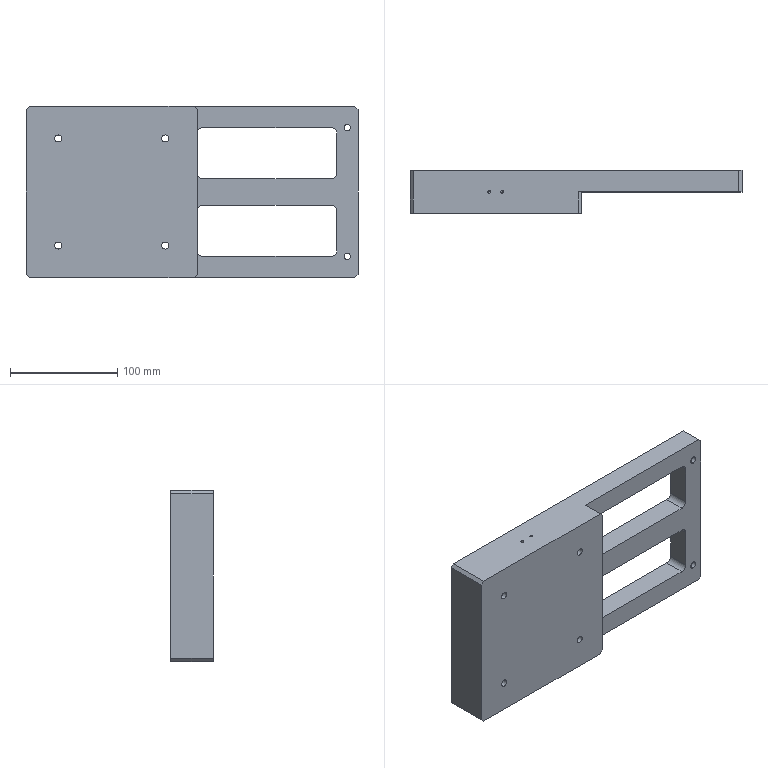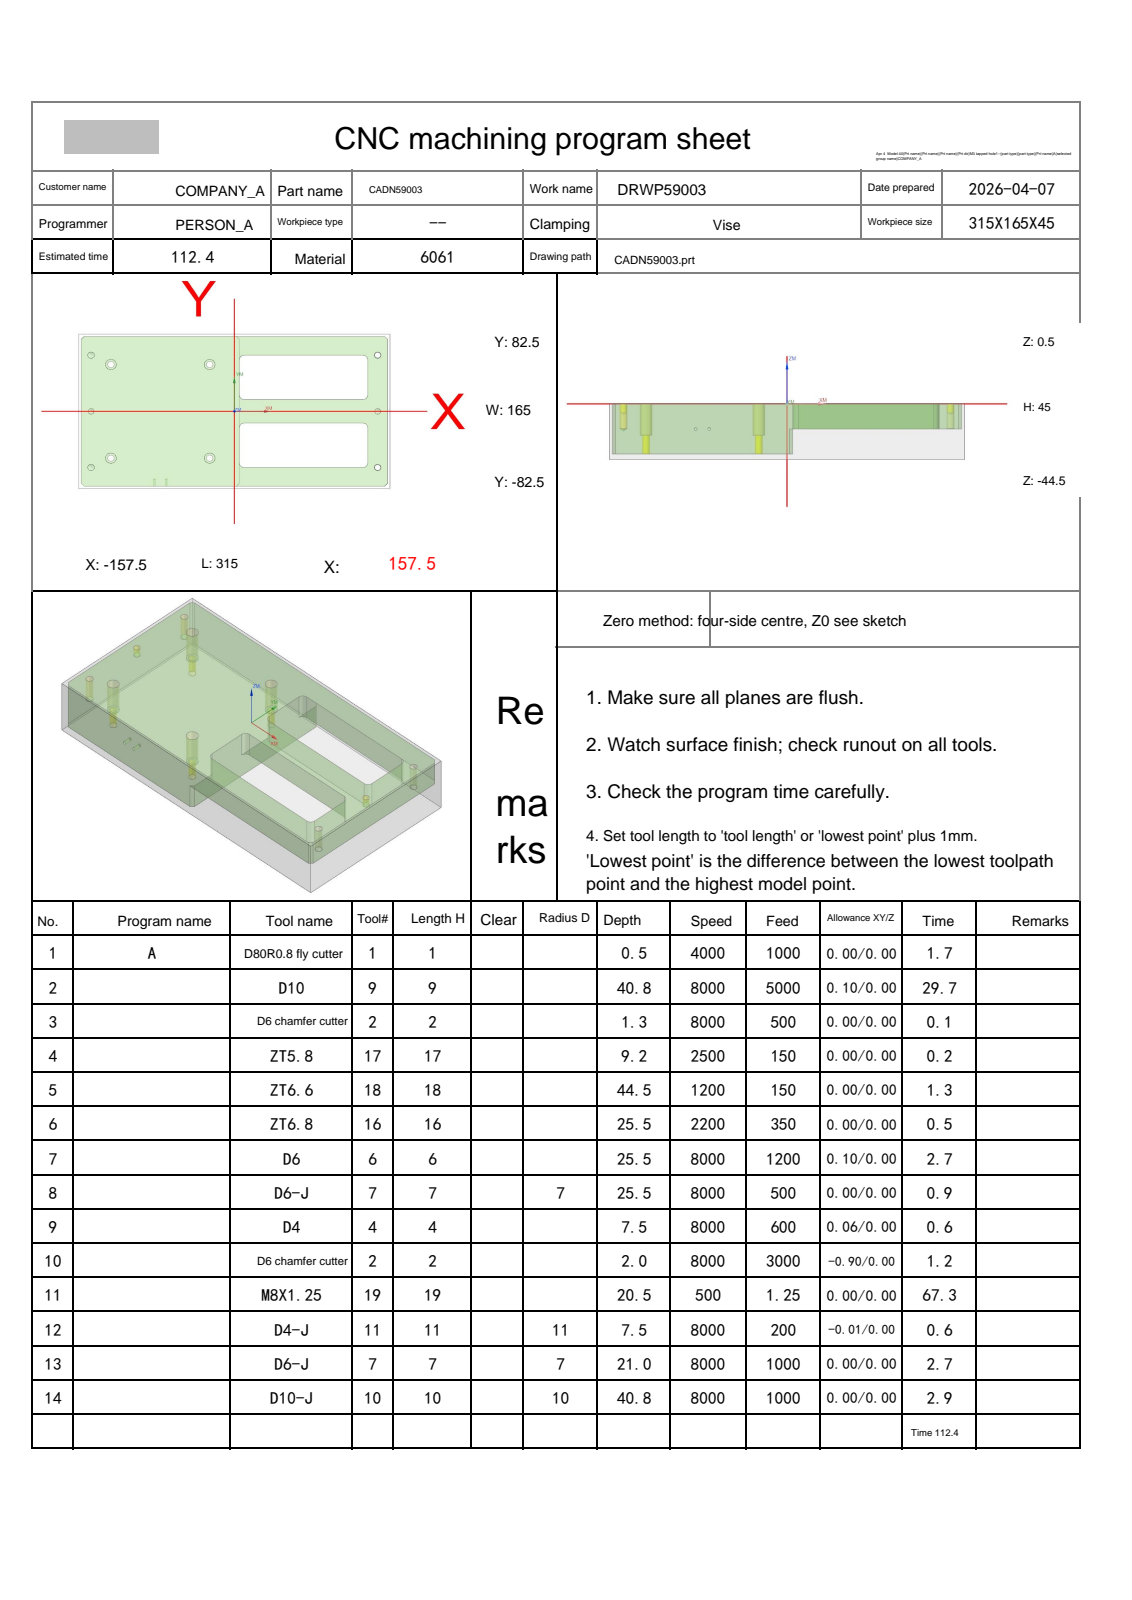NC program | NX | posted by the shop | part box 310 x 40 x 160 mm
Lines 4354 to 5464 of 5464:
N3 T02 M06
(D6 chamfer cutter  D=6. R=0. H=02 ce=0.00 di=0.10)
G00 G90 G54 X-145. Y-60. M03 S8000
G43 H02 Z20.
M08
G98 G81 X-145. Y-60. Z-.8 R1. F500.
X-125. Y-50.
X-145. Y0.0
Y60.
X-125. Y50.
X-25.
Y-50.
X145. Y-60.
Y0.0
Y60.
G80
G00 Z20.
G91 G28 Z0.0
M05
M09
G91 G28 Z0.0
M01
N4 T17 M06
(ZT5.8 D=5.8 DR_a=118 H=17)
G00 G90 G54 X-145. Y0.0 M03 S2500
G43 H17 Z20.
M08
G98 G83 X-145. Y0.0 Z-8.703 R1. F150. Q2.
X145.
G80
G00 Z20.
G91 G28 Z0.0
M05
M09
G91 G28 Z0.0
M01
N5 T18 M06
(ZT6.6 D=6.6 DR_a=118 H=18)
G00 G90 G54 X-25. Y50. M03 S1200
G43 H18 Z20.
M08
G98 G83 X-25. Y50. Z-43.983 R1. F150. Q2.
X-125.
Y-50.
X-25.
G80
G00 Z20.
G91 G28 Z0.0
M05
M09
G91 G28 Z0.0
M01
N6 T16 M06
(ZT6.8 D=6.8 DR_a=118 H=16)
G00 G90 G54 X-145. Y60. M03 S2200
G43 H16 Z20.
M08
G98 G83 X-145. Y60. Z-25. R1. F150. Q2.
Y-60.
G80
G00 Z20.
G00 G90 X145. Y-60. M03 S1800
Z20.
G98 G83 X145. Y-60. Z-25. R1. F350. Q3.
Y60.
G80
G00 Z20.
G91 G28 Z0.0
M05
M09
G91 G28 Z0.0
M01
N7 T06 M06
(D6  D=6. R=0. H=06 ce=0.10 di=0.00)
G00 G90 G54 X-25. Y50. M03 S8000
G43 H06 Z20.
M08
Z.5
G03 X-23.8 Y48.8 I1.2 J0.0 F1200.
X-22.6 Y50. I0.0 J1.2
X-22.6 Y50. Z0.0 I-2.4 J0.0
X-22.6 Y50. Z-.5 I-2.4 J0.0
X-22.6 Y50. Z-1. I-2.4 J0.0
X-22.6 Y50. Z-1.5 I-2.4 J0.0
X-22.6 Y50. Z-2. I-2.4 J0.0
X-22.6 Y50. Z-2.5 I-2.4 J0.0
X-22.6 Y50. Z-3. I-2.4 J0.0
X-22.6 Y50. Z-3.5 I-2.4 J0.0
X-22.6 Y50. Z-4. I-2.4 J0.0
X-22.6 Y50. Z-4.5 I-2.4 J0.0
X-22.6 Y50. Z-5. I-2.4 J0.0
X-22.6 Y50. Z-5.5 I-2.4 J0.0
X-22.6 Y50. Z-6. I-2.4 J0.0
X-22.6 Y50. Z-6.5 I-2.4 J0.0
X-22.6 Y50. Z-7. I-2.4 J0.0
X-22.6 Y50. Z-7.5 I-2.4 J0.0
X-22.6 Y50. Z-8. I-2.4 J0.0
X-22.6 Y50. Z-8.5 I-2.4 J0.0
X-22.6 Y50. Z-9. I-2.4 J0.0
X-22.6 Y50. Z-9.5 I-2.4 J0.0
X-22.6 Y50. Z-10. I-2.4 J0.0
X-22.6 Y50. Z-10.5 I-2.4 J0.0
X-22.6 Y50. Z-11. I-2.4 J0.0
X-22.6 Y50. Z-11.5 I-2.4 J0.0
X-22.6 Y50. Z-12. I-2.4 J0.0
X-22.6 Y50. Z-12.5 I-2.4 J0.0
X-22.6 Y50. Z-13. I-2.4 J0.0
X-22.6 Y50. Z-13.5 I-2.4 J0.0
X-22.6 Y50. Z-14. I-2.4 J0.0
X-22.6 Y50. Z-14.5 I-2.4 J0.0
X-22.6 Y50. Z-15. I-2.4 J0.0
X-22.6 Y50. Z-15.5 I-2.4 J0.0
X-22.6 Y50. Z-16. I-2.4 J0.0
X-22.6 Y50. Z-16.5 I-2.4 J0.0
X-22.6 Y50. Z-17. I-2.4 J0.0
X-22.6 Y50. Z-17.5 I-2.4 J0.0
X-22.6 Y50. Z-18. I-2.4 J0.0
X-22.6 Y50. Z-18.5 I-2.4 J0.0
X-22.6 Y50. Z-19. I-2.4 J0.0
X-22.6 Y50. Z-19.5 I-2.4 J0.0
X-22.6 Y50. Z-20. I-2.4 J0.0
X-22.6 Y50. Z-20.5 I-2.4 J0.0
X-22.6 Y50. Z-21. I-2.4 J0.0
X-22.6 Y50. Z-21.5 I-2.4 J0.0
X-22.6 Y50. Z-22. I-2.4 J0.0
X-22.6 Y50. Z-22.5 I-2.4 J0.0
X-22.6 Y50. Z-23. I-2.4 J0.0
X-22.6 Y50. Z-23.5 I-2.4 J0.0
X-22.6 Y50. Z-24. I-2.4 J0.0
X-22.6 Y50. Z-24.5 I-2.4 J0.0
X-22.6 Y50. Z-25. I-2.4 J0.0
X-25. Y52.4 I-2.4 J0.0
X-27.4 Y50. I0.0 J-2.4
X-25. Y47.6 I2.4 J0.0
X-22.6 Y50. I0.0 J2.4
X-23.8 Y51.2 I-1.2 J0.0
X-25. Y50. I0.0 J-1.2
G00 Z20.
X-125.
Z.5
G03 X-123.8 Y48.8 I1.2 J0.0
X-122.6 Y50. I0.0 J1.2
X-122.6 Y50. Z0.0 I-2.4 J0.0
X-122.6 Y50. Z-.5 I-2.4 J0.0
X-122.6 Y50. Z-1. I-2.4 J0.0
X-122.6 Y50. Z-1.5 I-2.4 J0.0
X-122.6 Y50. Z-2. I-2.4 J0.0
X-122.6 Y50. Z-2.5 I-2.4 J0.0
X-122.6 Y50. Z-3. I-2.4 J0.0
X-122.6 Y50. Z-3.5 I-2.4 J0.0
X-122.6 Y50. Z-4. I-2.4 J0.0
X-122.6 Y50. Z-4.5 I-2.4 J0.0
X-122.6 Y50. Z-5. I-2.4 J0.0
X-122.6 Y50. Z-5.5 I-2.4 J0.0
X-122.6 Y50. Z-6. I-2.4 J0.0
X-122.6 Y50. Z-6.5 I-2.4 J0.0
X-122.6 Y50. Z-7. I-2.4 J0.0
X-122.6 Y50. Z-7.5 I-2.4 J0.0
X-122.6 Y50. Z-8. I-2.4 J0.0
X-122.6 Y50. Z-8.5 I-2.4 J0.0
X-122.6 Y50. Z-9. I-2.4 J0.0
X-122.6 Y50. Z-9.5 I-2.4 J0.0
X-122.6 Y50. Z-10. I-2.4 J0.0
X-122.6 Y50. Z-10.5 I-2.4 J0.0
X-122.6 Y50. Z-11. I-2.4 J0.0
X-122.6 Y50. Z-11.5 I-2.4 J0.0
X-122.6 Y50. Z-12. I-2.4 J0.0
X-122.6 Y50. Z-12.5 I-2.4 J0.0
X-122.6 Y50. Z-13. I-2.4 J0.0
X-122.6 Y50. Z-13.5 I-2.4 J0.0
X-122.6 Y50. Z-14. I-2.4 J0.0
X-122.6 Y50. Z-14.5 I-2.4 J0.0
X-122.6 Y50. Z-15. I-2.4 J0.0
X-122.6 Y50. Z-15.5 I-2.4 J0.0
X-122.6 Y50. Z-16. I-2.4 J0.0
X-122.6 Y50. Z-16.5 I-2.4 J0.0
X-122.6 Y50. Z-17. I-2.4 J0.0
X-122.6 Y50. Z-17.5 I-2.4 J0.0
X-122.6 Y50. Z-18. I-2.4 J0.0
X-122.6 Y50. Z-18.5 I-2.4 J0.0
X-122.6 Y50. Z-19. I-2.4 J0.0
X-122.6 Y50. Z-19.5 I-2.4 J0.0
X-122.6 Y50. Z-20. I-2.4 J0.0
X-122.6 Y50. Z-20.5 I-2.4 J0.0
X-122.6 Y50. Z-21. I-2.4 J0.0
X-122.6 Y50. Z-21.5 I-2.4 J0.0
X-122.6 Y50. Z-22. I-2.4 J0.0
X-122.6 Y50. Z-22.5 I-2.4 J0.0
X-122.6 Y50. Z-23. I-2.4 J0.0
X-122.6 Y50. Z-23.5 I-2.4 J0.0
X-122.6 Y50. Z-24. I-2.4 J0.0
X-122.6 Y50. Z-24.5 I-2.4 J0.0
X-122.6 Y50. Z-25. I-2.4 J0.0
X-125. Y52.4 I-2.4 J0.0
X-127.4 Y50. I0.0 J-2.4
X-125. Y47.6 I2.4 J0.0
X-122.6 Y50. I0.0 J2.4
X-123.8 Y51.2 I-1.2 J0.0
X-125. Y50. I0.0 J-1.2
G00 Z20.
Y-50.
Z.5
G03 X-123.8 Y-51.2 I1.2 J0.0
X-122.6 Y-50. I0.0 J1.2
X-122.6 Y-50. Z0.0 I-2.4 J0.0
X-122.6 Y-50. Z-.5 I-2.4 J0.0
X-122.6 Y-50. Z-1. I-2.4 J0.0
X-122.6 Y-50. Z-1.5 I-2.4 J0.0
X-122.6 Y-50. Z-2. I-2.4 J0.0
X-122.6 Y-50. Z-2.5 I-2.4 J0.0
X-122.6 Y-50. Z-3. I-2.4 J0.0
X-122.6 Y-50. Z-3.5 I-2.4 J0.0
X-122.6 Y-50. Z-4. I-2.4 J0.0
X-122.6 Y-50. Z-4.5 I-2.4 J0.0
X-122.6 Y-50. Z-5. I-2.4 J0.0
X-122.6 Y-50. Z-5.5 I-2.4 J0.0
X-122.6 Y-50. Z-6. I-2.4 J0.0
X-122.6 Y-50. Z-6.5 I-2.4 J0.0
X-122.6 Y-50. Z-7. I-2.4 J0.0
X-122.6 Y-50. Z-7.5 I-2.4 J0.0
X-122.6 Y-50. Z-8. I-2.4 J0.0
X-122.6 Y-50. Z-8.5 I-2.4 J0.0
X-122.6 Y-50. Z-9. I-2.4 J0.0
X-122.6 Y-50. Z-9.5 I-2.4 J0.0
X-122.6 Y-50. Z-10. I-2.4 J0.0
X-122.6 Y-50. Z-10.5 I-2.4 J0.0
X-122.6 Y-50. Z-11. I-2.4 J0.0
X-122.6 Y-50. Z-11.5 I-2.4 J0.0
X-122.6 Y-50. Z-12. I-2.4 J0.0
X-122.6 Y-50. Z-12.5 I-2.4 J0.0
X-122.6 Y-50. Z-13. I-2.4 J0.0
X-122.6 Y-50. Z-13.5 I-2.4 J0.0
X-122.6 Y-50. Z-14. I-2.4 J0.0
X-122.6 Y-50. Z-14.5 I-2.4 J0.0
X-122.6 Y-50. Z-15. I-2.4 J0.0
X-122.6 Y-50. Z-15.5 I-2.4 J0.0
X-122.6 Y-50. Z-16. I-2.4 J0.0
X-122.6 Y-50. Z-16.5 I-2.4 J0.0
X-122.6 Y-50. Z-17. I-2.4 J0.0
X-122.6 Y-50. Z-17.5 I-2.4 J0.0
X-122.6 Y-50. Z-18. I-2.4 J0.0
X-122.6 Y-50. Z-18.5 I-2.4 J0.0
X-122.6 Y-50. Z-19. I-2.4 J0.0
X-122.6 Y-50. Z-19.5 I-2.4 J0.0
X-122.6 Y-50. Z-20. I-2.4 J0.0
X-122.6 Y-50. Z-20.5 I-2.4 J0.0
X-122.6 Y-50. Z-21. I-2.4 J0.0
X-122.6 Y-50. Z-21.5 I-2.4 J0.0
X-122.6 Y-50. Z-22. I-2.4 J0.0
X-122.6 Y-50. Z-22.5 I-2.4 J0.0
X-122.6 Y-50. Z-23. I-2.4 J0.0
X-122.6 Y-50. Z-23.5 I-2.4 J0.0
X-122.6 Y-50. Z-24. I-2.4 J0.0
X-122.6 Y-50. Z-24.5 I-2.4 J0.0
X-122.6 Y-50. Z-25. I-2.4 J0.0
X-125. Y-47.6 I-2.4 J0.0
X-127.4 Y-50. I0.0 J-2.4
X-125. Y-52.4 I2.4 J0.0
X-122.6 Y-50. I0.0 J2.4
X-123.8 Y-48.8 I-1.2 J0.0
X-125. Y-50. I0.0 J-1.2
G00 Z20.
X-25.
Z.5
G03 X-23.8 Y-51.2 I1.2 J0.0
X-22.6 Y-50. I0.0 J1.2
X-22.6 Y-50. Z0.0 I-2.4 J0.0
X-22.6 Y-50. Z-.5 I-2.4 J0.0
X-22.6 Y-50. Z-1. I-2.4 J0.0
X-22.6 Y-50. Z-1.5 I-2.4 J0.0
X-22.6 Y-50. Z-2. I-2.4 J0.0
X-22.6 Y-50. Z-2.5 I-2.4 J0.0
X-22.6 Y-50. Z-3. I-2.4 J0.0
X-22.6 Y-50. Z-3.5 I-2.4 J0.0
X-22.6 Y-50. Z-4. I-2.4 J0.0
X-22.6 Y-50. Z-4.5 I-2.4 J0.0
X-22.6 Y-50. Z-5. I-2.4 J0.0
X-22.6 Y-50. Z-5.5 I-2.4 J0.0
X-22.6 Y-50. Z-6. I-2.4 J0.0
X-22.6 Y-50. Z-6.5 I-2.4 J0.0
X-22.6 Y-50. Z-7. I-2.4 J0.0
X-22.6 Y-50. Z-7.5 I-2.4 J0.0
X-22.6 Y-50. Z-8. I-2.4 J0.0
X-22.6 Y-50. Z-8.5 I-2.4 J0.0
X-22.6 Y-50. Z-9. I-2.4 J0.0
X-22.6 Y-50. Z-9.5 I-2.4 J0.0
X-22.6 Y-50. Z-10. I-2.4 J0.0
X-22.6 Y-50. Z-10.5 I-2.4 J0.0
X-22.6 Y-50. Z-11. I-2.4 J0.0
X-22.6 Y-50. Z-11.5 I-2.4 J0.0
X-22.6 Y-50. Z-12. I-2.4 J0.0
X-22.6 Y-50. Z-12.5 I-2.4 J0.0
X-22.6 Y-50. Z-13. I-2.4 J0.0
X-22.6 Y-50. Z-13.5 I-2.4 J0.0
X-22.6 Y-50. Z-14. I-2.4 J0.0
X-22.6 Y-50. Z-14.5 I-2.4 J0.0
X-22.6 Y-50. Z-15. I-2.4 J0.0
X-22.6 Y-50. Z-15.5 I-2.4 J0.0
X-22.6 Y-50. Z-16. I-2.4 J0.0
X-22.6 Y-50. Z-16.5 I-2.4 J0.0
X-22.6 Y-50. Z-17. I-2.4 J0.0
X-22.6 Y-50. Z-17.5 I-2.4 J0.0
X-22.6 Y-50. Z-18. I-2.4 J0.0
X-22.6 Y-50. Z-18.5 I-2.4 J0.0
X-22.6 Y-50. Z-19. I-2.4 J0.0
X-22.6 Y-50. Z-19.5 I-2.4 J0.0
X-22.6 Y-50. Z-20. I-2.4 J0.0
X-22.6 Y-50. Z-20.5 I-2.4 J0.0
X-22.6 Y-50. Z-21. I-2.4 J0.0
X-22.6 Y-50. Z-21.5 I-2.4 J0.0
X-22.6 Y-50. Z-22. I-2.4 J0.0
X-22.6 Y-50. Z-22.5 I-2.4 J0.0
X-22.6 Y-50. Z-23. I-2.4 J0.0
X-22.6 Y-50. Z-23.5 I-2.4 J0.0
X-22.6 Y-50. Z-24. I-2.4 J0.0
X-22.6 Y-50. Z-24.5 I-2.4 J0.0
X-22.6 Y-50. Z-25. I-2.4 J0.0
X-25. Y-47.6 I-2.4 J0.0
X-27.4 Y-50. I0.0 J-2.4
X-25. Y-52.4 I2.4 J0.0
X-22.6 Y-50. I0.0 J2.4
X-23.8 Y-48.8 I-1.2 J0.0
X-25. Y-50. I0.0 J-1.2
G00 Z20.
G91 G28 Z0.0
M05
M09
G91 G28 Z0.0
M01
N8 T07 M06
(D6-J  D=6. R=0. H=07 ce=0.00 di=0.00)
G00 G90 G54 X-25. Y50. M03 S8000
G43 H07 Z20.
M08
Z0.0
G41 D07
G01 X-24.968 Y49.803 F500.
G03 X-23.742 Y48.758 I1.226 J.197
X-22.5 Y50. I0.0 J1.242
X-22.5 Y50. Z-5. I-2.5 J0.0
X-22.5 Y50. Z-10. I-2.5 J0.0
X-22.5 Y50. Z-15. I-2.5 J0.0
X-22.5 Y50. Z-20. I-2.5 J0.0
X-22.5 Y50. Z-25. I-2.5 J0.0
X-25. Y52.5 I-2.5 J0.0
X-27.5 Y50. I0.0 J-2.5
X-25. Y47.5 I2.5 J0.0
X-22.5 Y50. I0.0 J2.5
X-23.742 Y51.242 I-1.242 J0.0
X-24.968 Y50.197 I0.0 J-1.242
G01 G40 X-25. Y50.
G00 Z20.
X-125.
Z0.0
G41 D07
G01 X-124.968 Y49.803
G03 X-123.742 Y48.758 I1.226 J.197
X-122.5 Y50. I0.0 J1.242
X-122.5 Y50. Z-5. I-2.5 J0.0
X-122.5 Y50. Z-10. I-2.5 J0.0
X-122.5 Y50. Z-15. I-2.5 J0.0
X-122.5 Y50. Z-20. I-2.5 J0.0
X-122.5 Y50. Z-25. I-2.5 J0.0
X-125. Y52.5 I-2.5 J0.0
X-127.5 Y50. I0.0 J-2.5
X-125. Y47.5 I2.5 J0.0
X-122.5 Y50. I0.0 J2.5
X-123.742 Y51.242 I-1.242 J0.0
X-124.968 Y50.197 I0.0 J-1.242
G01 G40 X-125. Y50.
G00 Z20.
Y-50.
Z0.0
G41 D07
G01 X-124.968 Y-50.197
G03 X-123.742 Y-51.242 I1.226 J.197
X-122.5 Y-50. I0.0 J1.242
X-122.5 Y-50. Z-5. I-2.5 J0.0
X-122.5 Y-50. Z-10. I-2.5 J0.0
X-122.5 Y-50. Z-15. I-2.5 J0.0
X-122.5 Y-50. Z-20. I-2.5 J0.0
X-122.5 Y-50. Z-25. I-2.5 J0.0
X-125. Y-47.5 I-2.5 J0.0
X-127.5 Y-50. I0.0 J-2.5
X-125. Y-52.5 I2.5 J0.0
X-122.5 Y-50. I0.0 J2.5
X-123.742 Y-48.758 I-1.242 J0.0
X-124.968 Y-49.803 I0.0 J-1.242
G01 G40 X-125. Y-50.
G00 Z20.
X-25.
Z0.0
G41 D07
G01 X-24.968 Y-50.197
G03 X-23.742 Y-51.242 I1.226 J.197
X-22.5 Y-50. I0.0 J1.242
X-22.5 Y-50. Z-5. I-2.5 J0.0
X-22.5 Y-50. Z-10. I-2.5 J0.0
X-22.5 Y-50. Z-15. I-2.5 J0.0
X-22.5 Y-50. Z-20. I-2.5 J0.0
X-22.5 Y-50. Z-25. I-2.5 J0.0
X-25. Y-47.5 I-2.5 J0.0
X-27.5 Y-50. I0.0 J-2.5
X-25. Y-52.5 I2.5 J0.0
X-22.5 Y-50. I0.0 J2.5
X-23.742 Y-48.758 I-1.242 J0.0
X-24.968 Y-49.803 I0.0 J-1.242
G01 G40 X-25. Y-50.
G00 Z20.
G91 G28 Z0.0
M05
M09
G91 G28 Z0.0
M01
N9 T04 M06
(D4  D=4. R=0. H=04 ce=0.06 di=0.00)
G00 G90 G54 X-145. Y0.0 M03 S8000
G43 H04 Z20.
M08
Z.5
G03 X-144.53 Y-.47 I.47 J0.0 F600.
X-144.06 Y0.0 I0.0 J.47
X-144.06 Y0.0 Z.2 I-.94 J0.0
X-144.06 Y0.0 Z-.1 I-.94 J0.0
X-144.06 Y0.0 Z-.4 I-.94 J0.0
X-144.06 Y0.0 Z-.7 I-.94 J0.0
X-144.06 Y0.0 Z-1. I-.94 J0.0
X-144.06 Y0.0 Z-1.3 I-.94 J0.0
X-144.06 Y0.0 Z-1.6 I-.94 J0.0
X-144.06 Y0.0 Z-1.9 I-.94 J0.0
X-144.06 Y0.0 Z-2.2 I-.94 J0.0
X-144.06 Y0.0 Z-2.5 I-.94 J0.0
X-144.06 Y0.0 Z-2.8 I-.94 J0.0
X-144.06 Y0.0 Z-3.1 I-.94 J0.0
X-144.06 Y0.0 Z-3.4 I-.94 J0.0
X-144.06 Y0.0 Z-3.7 I-.94 J0.0
X-144.06 Y0.0 Z-4. I-.94 J0.0
X-144.06 Y0.0 Z-4.3 I-.94 J0.0
X-144.06 Y0.0 Z-4.6 I-.94 J0.0
X-144.06 Y0.0 Z-4.9 I-.94 J0.0
X-144.06 Y0.0 Z-5.2 I-.94 J0.0
X-144.06 Y0.0 Z-5.5 I-.94 J0.0
X-144.06 Y0.0 Z-5.8 I-.94 J0.0
X-144.06 Y0.0 Z-6.1 I-.94 J0.0
X-144.06 Y0.0 Z-6.4 I-.94 J0.0
X-144.06 Y0.0 Z-6.7 I-.94 J0.0
X-144.06 Y0.0 Z-7. I-.94 J0.0
X-145. Y.94 I-.94 J0.0
X-145.94 Y0.0 I0.0 J-.94
X-145. Y-.94 I.94 J0.0
X-144.06 Y0.0 I0.0 J.94
X-144.53 Y.47 I-.47 J0.0
X-145. Y0.0 I0.0 J-.47
G00 Z20.
X145.
Z.5
G03 X145.47 Y-.47 I.47 J0.0
X145.94 Y0.0 I0.0 J.47
X145.94 Y0.0 Z.2 I-.94 J0.0
X145.94 Y0.0 Z-.1 I-.94 J0.0
X145.94 Y0.0 Z-.4 I-.94 J0.0
X145.94 Y0.0 Z-.7 I-.94 J0.0
X145.94 Y0.0 Z-1. I-.94 J0.0
X145.94 Y0.0 Z-1.3 I-.94 J0.0
X145.94 Y0.0 Z-1.6 I-.94 J0.0
X145.94 Y0.0 Z-1.9 I-.94 J0.0
X145.94 Y0.0 Z-2.2 I-.94 J0.0
X145.94 Y0.0 Z-2.5 I-.94 J0.0
X145.94 Y0.0 Z-2.8 I-.94 J0.0
X145.94 Y0.0 Z-3.1 I-.94 J0.0
X145.94 Y0.0 Z-3.4 I-.94 J0.0
X145.94 Y0.0 Z-3.7 I-.94 J0.0
X145.94 Y0.0 Z-4. I-.94 J0.0
X145.94 Y0.0 Z-4.3 I-.94 J0.0
X145.94 Y0.0 Z-4.6 I-.94 J0.0
X145.94 Y0.0 Z-4.9 I-.94 J0.0
X145.94 Y0.0 Z-5.2 I-.94 J0.0
X145.94 Y0.0 Z-5.5 I-.94 J0.0
X145.94 Y0.0 Z-5.8 I-.94 J0.0
X145.94 Y0.0 Z-6.1 I-.94 J0.0
X145.94 Y0.0 Z-6.4 I-.94 J0.0
X145.94 Y0.0 Z-6.7 I-.94 J0.0
X145.94 Y0.0 Z-7. I-.94 J0.0
X145. Y.94 I-.94 J0.0
X144.06 Y0.0 I0.0 J-.94
X145. Y-.94 I.94 J0.0
X145.94 Y0.0 I0.0 J.94
X145.47 Y.47 I-.47 J0.0
X145. Y0.0 I0.0 J-.47
G00 Z20.
G91 G28 Z0.0
M05
M09
G91 G28 Z0.0
M01
N10 T02 M06
(D6 chamfer cutter  D=6. R=0. H=02 ce=0.00 di=0.00)
G00 G90 G54 X-.25 Y82.128 M03 S8000
G43 H02 Z20.
M08
Z2.099
G01 Z-1.5 F3000.
G03 X-.33 Y81.828 I.52 J-.3
X-.03 Y81.308 I.6 J0.0
G01 X0.0 Y81.3
X152.
X152.254 Y81.275
X152.497 Y81.201
X152.722 Y81.081
X152.919 Y80.919
X155.919 Y77.919
X156.081 Y77.722
X156.201 Y77.497
X156.275 Y77.254
X156.3 Y77.
Y-77.
X156.275 Y-77.254
X156.201 Y-77.497
X156.081 Y-77.722
X155.919 Y-77.919
X152.919 Y-80.919
X152.722 Y-81.081
X152.497 Y-81.201
X152.254 Y-81.275
X152. Y-81.3
X-152.
X-152.254 Y-81.275
X-152.497 Y-81.201
X-152.722 Y-81.081
X-152.919 Y-80.919
X-155.919 Y-77.919
X-156.081 Y-77.722
X-156.201 Y-77.497
X-156.275 Y-77.254
X-156.3 Y-77.
Y77.
X-156.275 Y77.254
X-156.201 Y77.497
X-156.081 Y77.722
X-155.919 Y77.919
X-152.919 Y80.919
X-152.722 Y81.081
X-152.497 Y81.201
X-152.254 Y81.275
X-152. Y81.3
X0.0
X.03 Y81.308
G03 X.33 Y81.828 I-.3 J.52
X.25 Y82.128 I-.6 J0.0
G01 Z2.099
G00 Z20.
X69.75 Y14.628
Z2.099
G01 Z-1.5
G03 X69.67 Y14.328 I.52 J-.3
X69.97 Y13.808 I.6 J0.0
G01 X70. Y13.8
X130.
G03 X133.7 Y17.5 I0.0 J3.7
G01 Y55.
G03 X130. Y58.7 I-3.7 J0.0
G01 X10.
G03 X6.3 Y55. I0.0 J-3.7
G01 Y17.5
G03 X10. Y13.8 I3.7 J0.0
G01 X70.
X70.03 Y13.808
G03 X70.33 Y14.328 I-.3 J.52
X70.25 Y14.628 I-.6 J0.0
G01 Z2.099
G00 Z20.
Y-14.628
Z2.099
G01 Z-1.5
G03 X70.33 Y-14.328 I-.52 J.3
X70.03 Y-13.808 I-.6 J0.0
G01 X70. Y-13.8
X10.
G03 X6.3 Y-17.5 I0.0 J-3.7
G01 Y-55.
G03 X10. Y-58.7 I3.7 J0.0
G01 X130.
G03 X133.7 Y-55. I0.0 J3.7
G01 Y-17.5
G03 X130. Y-13.8 I-3.7 J0.0
G01 X70.
X69.97 Y-13.808
G03 X69.67 Y-14.328 I.3 J-.52
X69.75 Y-14.628 I.6 J0.0
G01 Z2.099
G00 Z20.
G00 G90 X-146.147 Y-.612 M03 S8000
Z20.
Z-.5
G01 Z-1. F500.
X-146.5 Y-.8
G03 X-145. Y-2.3 I1.5 J0.0
X-142.7 Y0.0 I0.0 J2.3
X-145. Y2.3 I-2.3 J0.0
X-147.3 Y0.0 I0.0 J-2.3
X-145. Y-2.3 I2.3 J0.0
X-143.5 Y-.8 I0.0 J1.5
G01 X-143.853 Y-.612
Z-.5
G00 Z20.
X143.853
Z-.5
G01 Z-1.
X143.5 Y-.8
G03 X145. Y-2.3 I1.5 J0.0
X147.3 Y0.0 I0.0 J2.3
X145. Y2.3 I-2.3 J0.0
X142.7 Y0.0 I0.0 J-2.3
X145. Y-2.3 I2.3 J0.0
X146.5 Y-.8 I0.0 J1.5
G01 X146.147 Y-.612
Z-.5
G00 Z20.
G00 G90 X143. Y60. M03 S8000
Z20.
Z-.7
G01 Z-1.2 F600.
X142.
G03 X145. Y57. I3. J0.0
X148. Y60. I0.0 J3.
X145. Y63. I-3. J0.0
X142. Y60. I0.0 J-3.
X145. Y57. I3. J0.0
X148. Y60. I0.0 J3.
G01 X147.
Z-.7
G00 Z20.
X143. Y-60.
Z-.7
G01 Z-1.2
X142.
G03 X145. Y-63. I3. J0.0
X148. Y-60. I0.0 J3.
X145. Y-57. I-3. J0.0
X142. Y-60. I0.0 J-3.
X145. Y-63. I3. J0.0
X148. Y-60. I0.0 J3.
G01 X147.
Z-.7
G00 Z20.
G00 G90 X-146.5 Y58.834 M03 S8000
Z20.
Z-.9
G01 Z-1.4 F600.
Y58.6
G03 X-145. Y57.1 I1.5 J0.0
X-142.1 Y60. I0.0 J2.9
X-145. Y62.9 I-2.9 J0.0
X-147.9 Y60. I0.0 J-2.9
X-145. Y57.1 I2.9 J0.0
X-143.5 Y58.6 I0.0 J1.5
G01 Y58.834
Z-.9
G00 Z20.
X-146.5 Y-61.166
Z-.9
G01 Z-1.4
Y-61.4
G03 X-145. Y-62.9 I1.5 J0.0
X-142.1 Y-60. I0.0 J2.9
X-145. Y-57.1 I-2.9 J0.0
X-147.9 Y-60. I0.0 J-2.9
X-145. Y-62.9 I2.9 J0.0
X-143.5 Y-61.4 I0.0 J1.5
G01 Y-61.166
Z-.9
G00 Z20.
G00 G90 X-20.643 Y-52.009 M03 S8000
Z20.
Z2.5
G01 X-20.561 Y-51.834 Z2.43 F800.
X-20.405 Y-51.399 Z2.261
X-20.292 Y-50.95 Z2.093
X-20.222 Y-50.493 Z1.925
X-20.197 Y-50.031 Z1.756
X-20.216 Y-49.569 Z1.588
X-20.28 Y-49.11 Z1.419
X-20.388 Y-48.66 Z1.251
X-20.538 Y-48.223 Z1.083
X-20.73 Y-47.802 Z.914
X-20.961 Y-47.401 Z.746
X-21.23 Y-47.024 Z.577
X-21.534 Y-46.675 Z.409
X-21.87 Y-46.357 Z.241
X-22.235 Y-46.073 Z.072
X-22.625 Y-45.825 Z-.096
X-23.038 Y-45.616 Z-.265
X-23.469 Y-45.448 Z-.433
X-23.914 Y-45.321 Z-.601
X-24.369 Y-45.239 Z-.77
X-24.83 Y-45.2 Z-.938
X-25. Z-1.
G03 X-29.8 Y-50. I0.0 J-4.8
X-25. Y-54.8 I4.8 J0.0
X-20.2 Y-50. I0.0 J4.8
X-25. Y-45.2 I-4.8 J0.0
X-25.499 Y-45.226 I0.0 J-4.8
G01 Z1.5
G00 Z20.
X-120.643 Y-52.009
Z2.5
G01 X-120.561 Y-51.834 Z2.43
X-120.405 Y-51.399 Z2.261
X-120.292 Y-50.95 Z2.093
X-120.222 Y-50.493 Z1.925
X-120.197 Y-50.031 Z1.756
X-120.216 Y-49.569 Z1.588
X-120.28 Y-49.11 Z1.419
X-120.388 Y-48.66 Z1.251
X-120.538 Y-48.223 Z1.083
X-120.73 Y-47.802 Z.914
X-120.961 Y-47.401 Z.746
X-121.23 Y-47.024 Z.577
X-121.534 Y-46.675 Z.409
X-121.87 Y-46.357 Z.241
X-122.235 Y-46.073 Z.072
X-122.625 Y-45.825 Z-.096
X-123.038 Y-45.616 Z-.265
X-123.469 Y-45.448 Z-.433
X-123.914 Y-45.321 Z-.601
X-124.369 Y-45.239 Z-.77
X-124.83 Y-45.2 Z-.938
X-125. Z-1.
G03 X-129.8 Y-50. I0.0 J-4.8
X-125. Y-54.8 I4.8 J0.0
X-120.2 Y-50. I0.0 J4.8
X-125. Y-45.2 I-4.8 J0.0
X-125.499 Y-45.226 I0.0 J-4.8
G01 Z1.5
G00 Z20.
X-120.643 Y47.991
Z2.5
G01 X-120.561 Y48.166 Z2.43
X-120.405 Y48.601 Z2.261
X-120.292 Y49.05 Z2.093
X-120.222 Y49.507 Z1.925
X-120.197 Y49.969 Z1.756
X-120.216 Y50.431 Z1.588
X-120.28 Y50.89 Z1.419
X-120.388 Y51.34 Z1.251
X-120.538 Y51.777 Z1.083
X-120.73 Y52.198 Z.914
X-120.961 Y52.599 Z.746
X-121.23 Y52.976 Z.577
X-121.534 Y53.325 Z.409
X-121.87 Y53.643 Z.241
X-122.235 Y53.927 Z.072
X-122.625 Y54.175 Z-.096
X-123.038 Y54.384 Z-.265
X-123.469 Y54.552 Z-.433
X-123.914 Y54.679 Z-.601
X-124.369 Y54.761 Z-.77
X-124.83 Y54.8 Z-.938
X-125. Z-1.
G03 X-129.8 Y50. I0.0 J-4.8
X-125. Y45.2 I4.8 J0.0
X-120.2 Y50. I0.0 J4.8
X-125. Y54.8 I-4.8 J0.0
X-125.499 Y54.774 I0.0 J-4.8
G01 Z1.5
G00 Z20.
X-20.643 Y47.991
Z2.5
G01 X-20.561 Y48.166 Z2.43
X-20.405 Y48.601 Z2.261
X-20.292 Y49.05 Z2.093
X-20.222 Y49.507 Z1.925
X-20.197 Y49.969 Z1.756
X-20.216 Y50.431 Z1.588
X-20.28 Y50.89 Z1.419
X-20.388 Y51.34 Z1.251
X-20.538 Y51.777 Z1.083
X-20.73 Y52.198 Z.914
X-20.961 Y52.599 Z.746
X-21.23 Y52.976 Z.577
X-21.534 Y53.325 Z.409
X-21.87 Y53.643 Z.241
X-22.235 Y53.927 Z.072
X-22.625 Y54.175 Z-.096
X-23.038 Y54.384 Z-.265
X-23.469 Y54.552 Z-.433
X-23.914 Y54.679 Z-.601
X-24.369 Y54.761 Z-.77
X-24.83 Y54.8 Z-.938
X-25. Z-1.
G03 X-29.8 Y50. I0.0 J-4.8
X-25. Y45.2 I4.8 J0.0
X-20.2 Y50. I0.0 J4.8
X-25. Y54.8 I-4.8 J0.0
X-25.499 Y54.774 I0.0 J-4.8
G01 Z1.5
G00 Z20.
G91 G28 Z0.0
M05
M09
G91 G28 Z0.0
M01
N11 T19 M06
(M8X1.25 D=6.8 DR_a=180 H=19)
G00 G90 G54 X145. Y60. M03 S500
G43 H19 Z20.
M08
G95
G98 G84 X145. Y60. Z-20. R1. F1.25 Q4.
Y-60.
X-145.
Y60.
G80
G94
G00 Z20.
G91 G28 Z0.0
M05
M09
G91 G28 Z0.0
M01
N12 T11 M06
(D4-J  D=4. R=0. H=11 ce=-0.01 di=0.00)
G00 G90 G54 X-145. Y0.0 M03 S8000
G43 H11 Z20.
M08
Z.5
G41 D11
G01 X-144.924 Y-.185 F200.
G03 X-144.475 Y-.485 I.449 J.185
X-143.99 Y0.0 I0.0 J.485
X-143.99 Y0.0 Z-.5 I-1.01 J0.0
X-143.99 Y0.0 Z-1.5 I-1.01 J0.0
X-143.99 Y0.0 Z-2.5 I-1.01 J0.0
X-143.99 Y0.0 Z-3.5 I-1.01 J0.0
X-143.99 Y0.0 Z-4.5 I-1.01 J0.0
X-143.99 Y0.0 Z-5.5 I-1.01 J0.0
X-143.99 Y0.0 Z-6.5 I-1.01 J0.0
X-146.01 Y0.0 Z-7. I-1.01 J0.0
X-145. Y-1.01 I1.01 J0.0
X-143.99 Y0.0 I0.0 J1.01
X-145. Y1.01 I-1.01 J0.0
X-146.01 Y0.0 I0.0 J-1.01
X-145.525 Y-.485 I.485 J0.0
X-145.076 Y-.185 I0.0 J.485
G01 G40 X-145. Y0.0
G00 Z20.
X145.
Z.5
G41 D11
G01 X145.076 Y-.185
G03 X145.525 Y-.485 I.449 J.185
X146.01 Y0.0 I0.0 J.485
X146.01 Y0.0 Z-.5 I-1.01 J0.0
X146.01 Y0.0 Z-1.5 I-1.01 J0.0
X146.01 Y0.0 Z-2.5 I-1.01 J0.0
X146.01 Y0.0 Z-3.5 I-1.01 J0.0
X146.01 Y0.0 Z-4.5 I-1.01 J0.0
X146.01 Y0.0 Z-5.5 I-1.01 J0.0
X146.01 Y0.0 Z-6.5 I-1.01 J0.0
X143.99 Y0.0 Z-7. I-1.01 J0.0
X145. Y-1.01 I1.01 J0.0
X146.01 Y0.0 I0.0 J1.01
X145. Y1.01 I-1.01 J0.0
X143.99 Y0.0 I0.0 J-1.01
X144.475 Y-.485 I.485 J0.0
X144.924 Y-.185 I0.0 J.485
G01 G40 X145. Y0.0
G00 Z20.
G91 G28 Z0.0
M05
M09
G91 G28 Z0.0
M01
N13 T07 M06
(D6-J  D=6. R=0. H=07 ce=0.00 di=0.00)
G00 G90 G54 X130.9 Y55.432 M03 S8000
G43 H07 Z5.5
M08
Z-4.125
G01 Z-5.125 F1000.
G41 D07
Y56.1
G03 X130. Y57. I-.9 J0.0
G01 X10.
G03 X8. Y55. I0.0 J-2.
G01 Y17.5
G03 X10. Y15.5 I2. J0.0
G01 X130.
G03 X132. Y17.5 I0.0 J2.
G01 Y55.
G03 X130. Y57. I-2. J0.0
X129.1 Y56.1 I0.0 J-.9
G01 G40 Y55.9
Z-4.125
G00 X130.9 Y55.432
Z-9.25
G01 Z-10.25
G41 D07
Y56.1
G03 X130. Y57. I-.9 J0.0
G01 X10.
G03 X8. Y55. I0.0 J-2.
G01 Y17.5
G03 X10. Y15.5 I2. J0.0
G01 X130.
G03 X132. Y17.5 I0.0 J2.
G01 Y55.
G03 X130. Y57. I-2. J0.0
X129.1 Y56.1 I0.0 J-.9
G01 G40 Y55.9
Z-9.25
G00 X130.9 Y55.432
Z-14.375
G01 Z-15.375
G41 D07
Y56.1
G03 X130. Y57. I-.9 J0.0
G01 X10.
G03 X8. Y55. I0.0 J-2.
G01 Y17.5
G03 X10. Y15.5 I2. J0.0
G01 X130.
G03 X132. Y17.5 I0.0 J2.
G01 Y55.
G03 X130. Y57. I-2. J0.0
X129.1 Y56.1 I0.0 J-.9
G01 G40 Y55.9
Z-14.375
G00 X130.9 Y55.432
Z-19.5
G01 Z-20.5
G41 D07
Y56.1
G03 X130. Y57. I-.9 J0.0
G01 X10.
G03 X8. Y55. I0.0 J-2.
G01 Y17.5
G03 X10. Y15.5 I2. J0.0
G01 X130.
G03 X132. Y17.5 I0.0 J2.
G01 Y55.
G03 X130. Y57. I-2. J0.0
X129.1 Y56.1 I0.0 J-.9
G01 G40 Y55.9
Z-19.5
G00 Z5.5
X9.1 Y-55.432
Z-4.125
G01 Z-5.125
G41 D07
Y-56.1
G03 X10. Y-57. I.9 J0.0
G01 X130.
G03 X132. Y-55. I0.0 J2.
G01 Y-17.5
G03 X130. Y-15.5 I-2. J0.0
G01 X10.
G03 X8. Y-17.5 I0.0 J-2.
G01 Y-55.
G03 X10. Y-57. I2. J0.0
X10.9 Y-56.1 I0.0 J.9
G01 G40 Y-55.9
Z-4.125
G00 X9.1 Y-55.432
Z-9.25
G01 Z-10.25
G41 D07
Y-56.1
G03 X10. Y-57. I.9 J0.0
G01 X130.
G03 X132. Y-55. I0.0 J2.
G01 Y-17.5
G03 X130. Y-15.5 I-2. J0.0
G01 X10.
G03 X8. Y-17.5 I0.0 J-2.
G01 Y-55.
G03 X10. Y-57. I2. J0.0
X10.9 Y-56.1 I0.0 J.9
G01 G40 Y-55.9
Z-9.25
G00 X9.1 Y-55.432
Z-14.375
G01 Z-15.375
G41 D07
Y-56.1
G03 X10. Y-57. I.9 J0.0
G01 X130.
G03 X132. Y-55. I0.0 J2.
G01 Y-17.5
G03 X130. Y-15.5 I-2. J0.0
G01 X10.
G03 X8. Y-17.5 I0.0 J-2.
G01 Y-55.
G03 X10. Y-57. I2. J0.0
X10.9 Y-56.1 I0.0 J.9
G01 G40 Y-55.9
Z-14.375
G00 X9.1 Y-55.432
Z-19.5
G01 Z-20.5
G41 D07
Y-56.1
G03 X10. Y-57. I.9 J0.0
G01 X130.
G03 X132. Y-55. I0.0 J2.
G01 Y-17.5
G03 X130. Y-15.5 I-2. J0.0
G01 X10.
G03 X8. Y-17.5 I0.0 J-2.
G01 Y-55.
G03 X10. Y-57. I2. J0.0
X10.9 Y-56.1 I0.0 J.9
G01 G40 Y-55.9
Z-19.5
G00 Z5.5
G91 G28 Z0.0
M05
M09
G91 G28 Z0.0
M01
N14 T10 M06
(D10-J  D=10. R=0. H=10 ce=0.00 di=0.00)
G00 G90 G54 X-153.013 Y86.116 M03 S8000
G43 H10 Z20.
M08
Z-12.933
G01 Z-13.433 F1000.
G41 D10
X-152.997 Y85.917
G03 X-152. Y85. I.997 J.083
G01 X152.
G02 X155.536 Y83.536 I0.0 J-5.
G01 X158.536 Y80.536
G02 X160. Y77. I-3.536 J-3.536
G01 Y-77.
G02 X158.536 Y-80.536 I-5. J0.0
G01 X155.536 Y-83.536
G02 X152. Y-85. I-3.536 J3.536
G01 X-152.
G02 X-155.536 Y-83.536 I0.0 J5.
G01 X-158.536 Y-80.536
G02 X-160. Y-77. I3.536 J3.536
G01 Y77.
G02 X-158.536 Y80.536 I5. J0.0
G01 X-155.536 Y83.536
G02 X-152. Y85. I3.536 J-3.536
G01 X-151.5
G03 X-150.5 Y86. I0.0 J1.
G01 G40 Y86.2
Z-12.933
G00 Z20.
X-153.013 Y86.116
Z-26.367
G01 Z-26.867
G41 D10
X-152.997 Y85.917
G03 X-152. Y85. I.997 J.083
G01 X152.
G02 X155.536 Y83.536 I0.0 J-5.
G01 X158.536 Y80.536
G02 X160. Y77. I-3.536 J-3.536
G01 Y-77.
G02 X158.536 Y-80.536 I-5. J0.0
G01 X155.536 Y-83.536
G02 X152. Y-85. I-3.536 J3.536
G01 X-152.
G02 X-155.536 Y-83.536 I0.0 J5.
G01 X-158.536 Y-80.536
G02 X-160. Y-77. I3.536 J3.536
G01 Y77.
G02 X-158.536 Y80.536 I5. J0.0
G01 X-155.536 Y83.536
G02 X-152. Y85. I3.536 J-3.536
G01 X-151.5
G03 X-150.5 Y86. I0.0 J1.
G01 G40 Y86.2
Z-26.367
G00 Z20.
X-153.013 Y86.116
Z-39.8
G01 Z-40.3
G41 D10
X-152.997 Y85.917
G03 X-152. Y85. I.997 J.083
G01 X152.
G02 X155.536 Y83.536 I0.0 J-5.
G01 X158.536 Y80.536
G02 X160. Y77. I-3.536 J-3.536
G01 Y-77.
G02 X158.536 Y-80.536 I-5. J0.0
G01 X155.536 Y-83.536
G02 X152. Y-85. I-3.536 J3.536
G01 X-152.
G02 X-155.536 Y-83.536 I0.0 J5.
G01 X-158.536 Y-80.536
G02 X-160. Y-77. I3.536 J3.536
G01 Y77.
G02 X-158.536 Y80.536 I5. J0.0
G01 X-155.536 Y83.536
G02 X-152. Y85. I3.536 J-3.536
G01 X-151.5
G03 X-150.5 Y86. I0.0 J1.
G01 G40 Y86.2
Z-39.8
G00 Z20.
M05
M09
G91 G28 Z0.0
G91 G28 Y0.0
M30
%